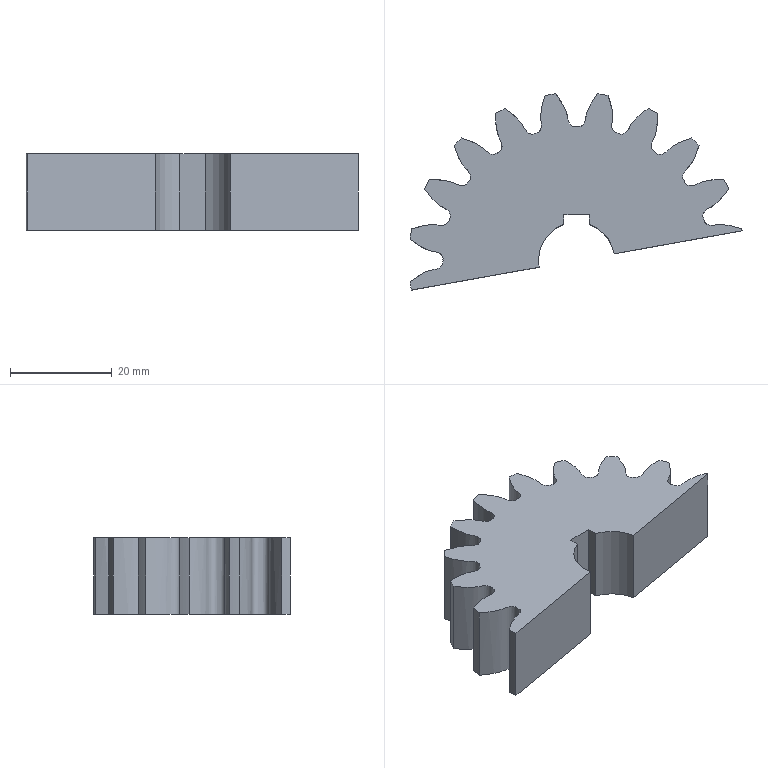Part | STEP file | Cuon T phu H01_5_Spur01 | 1 solid | 30 faces | box 65.224 x 38.555 x 15 mm | volume 19544 mm3 | cylinder 13 | spline 10 | plane 7 | commonest cylinder face diameters 66 x11 15 x2